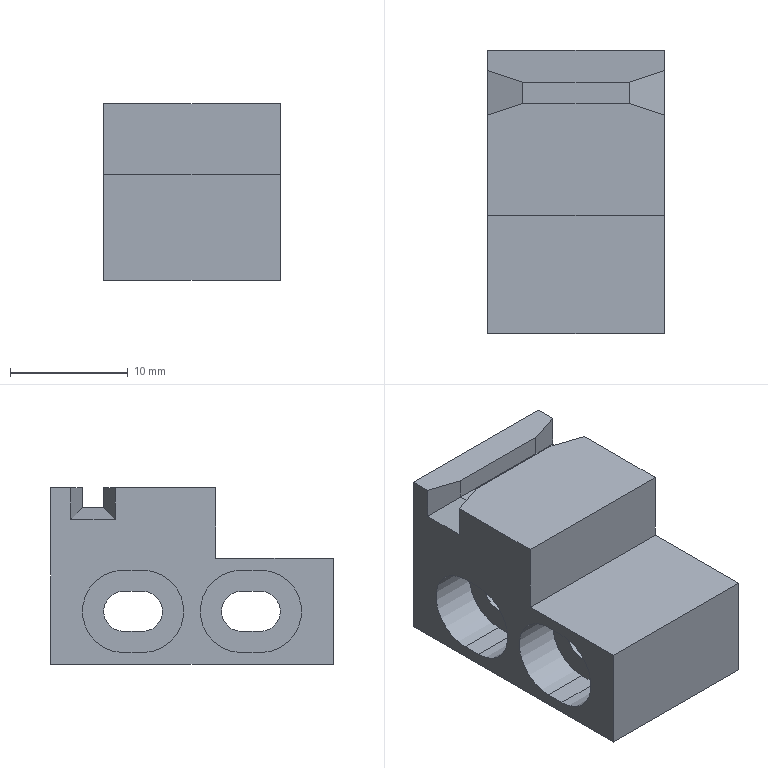Part | NX | features BREP 1 | 1 solid | 48 faces | box 15 x 24 x 15 mm | volume 3436 mm3 | plane 34 | cylinder 14 | commonest cylinder face diameters 7 x10 3.4 x4
STEP:
#1=CARTESIAN_POINT('',(-8.,-13.5,1.5));
#2=VERTEX_POINT('',#1);
#3=CARTESIAN_POINT('',(-8.,-3.5,1.5));
#4=VERTEX_POINT('',#3);
#5=CARTESIAN_POINT('',(-8.,-13.5,1.5));
#6=DIRECTION('',(0.,1.,0.));
#7=VECTOR('',#6,1000.);
#8=LINE('',#5,#7);
#9=EDGE_CURVE('',#2,#4,#8,.T.);
#10=ORIENTED_EDGE('',*,*,#9,.T.);
#11=CARTESIAN_POINT('',(-23.,-3.5,1.5));
#12=VERTEX_POINT('',#11);
#13=CARTESIAN_POINT('',(-23.,-3.5,1.5));
#14=DIRECTION('',(1.,0.,0.));
#15=VECTOR('',#14,1000.);
#16=LINE('',#13,#15);
#17=EDGE_CURVE('',#12,#4,#16,.T.);
#18=ORIENTED_EDGE('',*,*,#17,.F.);
#19=CARTESIAN_POINT('',(-23.,-13.5,1.5));
#20=VERTEX_POINT('',#19);
#21=CARTESIAN_POINT('',(-23.,-13.5,1.5));
#22=DIRECTION('',(0.,1.,0.));
#23=VECTOR('',#22,1000.);
#24=LINE('',#21,#23);
#25=EDGE_CURVE('',#20,#12,#24,.T.);
#26=ORIENTED_EDGE('',*,*,#25,.F.);
#27=CARTESIAN_POINT('',(-23.,-13.5,1.5));
#28=DIRECTION('',(1.,0.,0.));
#29=VECTOR('',#28,1000.);
#30=LINE('',#27,#29);
#31=EDGE_CURVE('',#20,#2,#30,.T.);
#32=ORIENTED_EDGE('',*,*,#31,.T.);
#33=EDGE_LOOP('',(#10,#18,#26,#32));
#34=FACE_BOUND('',#33,.T.);
#35=CARTESIAN_POINT('',(-23.,-13.5,1.5));
#36=DIRECTION('',(0.,0.,-1.));
#37=DIRECTION('',(-1.,0.,0.));
#38=AXIS2_PLACEMENT_3D('',#35,#36,#37);
#39=PLANE('',#38);
#40=ADVANCED_FACE('',(#34),#39,.F.);
#41=CARTESIAN_POINT('',(-8.,-3.5,7.5));
#42=VERTEX_POINT('',#41);
#43=CARTESIAN_POINT('',(-8.,-3.5,7.5));
#44=DIRECTION('',(0.,0.,1.));
#45=VECTOR('',#44,1000.);
#46=LINE('',#43,#45);
#47=EDGE_CURVE('',#4,#42,#46,.T.);
#48=ORIENTED_EDGE('',*,*,#47,.T.);
#49=CARTESIAN_POINT('',(-23.,-3.5,7.5));
#50=VERTEX_POINT('',#49);
#51=CARTESIAN_POINT('',(-23.,-3.5,7.5));
#52=DIRECTION('',(1.,0.,0.));
#53=VECTOR('',#52,1000.);
#54=LINE('',#51,#53);
#55=EDGE_CURVE('',#50,#42,#54,.T.);
#56=ORIENTED_EDGE('',*,*,#55,.F.);
#57=CARTESIAN_POINT('',(-23.,-3.5,7.5));
#58=DIRECTION('',(0.,0.,1.));
#59=VECTOR('',#58,1000.);
#60=LINE('',#57,#59);
#61=EDGE_CURVE('',#12,#50,#60,.T.);
#62=ORIENTED_EDGE('',*,*,#61,.F.);
#63=ORIENTED_EDGE('',*,*,#17,.T.);
#64=EDGE_LOOP('',(#48,#56,#62,#63));
#65=FACE_BOUND('',#64,.T.);
#66=CARTESIAN_POINT('',(-23.,-3.5,7.5));
#67=DIRECTION('',(0.,1.,0.));
#68=DIRECTION('',(-1.,0.,0.));
#69=AXIS2_PLACEMENT_3D('',#66,#67,#68);
#70=PLANE('',#69);
#71=ADVANCED_FACE('',(#65),#70,.F.);
#72=CARTESIAN_POINT('',(-8.,5.,4.8));
#73=VERTEX_POINT('',#72);
#74=CARTESIAN_POINT('',(-11.,6.,5.8));
#75=VERTEX_POINT('',#74);
#76=CARTESIAN_POINT('',(-8.736,5.245,5.045));
#77=DIRECTION('',(-0.9045,0.3015,0.3015));
#78=VECTOR('',#77,1000.);
#79=LINE('',#76,#78);
#80=EDGE_CURVE('',#73,#75,#79,.T.);
#81=ORIENTED_EDGE('',*,*,#80,.T.);
#82=CARTESIAN_POINT('',(-11.,6.,7.5));
#83=VERTEX_POINT('',#82);
#84=CARTESIAN_POINT('',(-11.,6.,5.8));
#85=DIRECTION('',(0.,0.,-1.));
#86=VECTOR('',#85,1000.);
#87=LINE('',#84,#86);
#88=EDGE_CURVE('',#83,#75,#87,.T.);
#89=ORIENTED_EDGE('',*,*,#88,.F.);
#90=CARTESIAN_POINT('',(-8.,5.,7.5));
#91=VERTEX_POINT('',#90);
#92=CARTESIAN_POINT('',(-8.,5.,7.5));
#93=DIRECTION('',(-0.9487,0.3162,0.));
#94=VECTOR('',#93,1000.);
#95=LINE('',#92,#94);
#96=EDGE_CURVE('',#91,#83,#95,.T.);
#97=ORIENTED_EDGE('',*,*,#96,.F.);
#98=CARTESIAN_POINT('',(-8.,5.,7.5));
#99=DIRECTION('',(0.,0.,1.));
#100=VECTOR('',#99,1000.);
#101=LINE('',#98,#100);
#102=EDGE_CURVE('',#73,#91,#101,.T.);
#103=ORIENTED_EDGE('',*,*,#102,.F.);
#104=EDGE_LOOP('',(#81,#89,#97,#103));
#105=FACE_BOUND('',#104,.T.);
#106=CARTESIAN_POINT('',(-8.,5.,7.5));
#107=DIRECTION('',(-0.3162,-0.9487,0.));
#108=DIRECTION('',(0.,0.,1.));
#109=AXIS2_PLACEMENT_3D('',#106,#107,#108);
#110=PLANE('',#109);
#111=ADVANCED_FACE('',(#105),#110,.F.);
#112=CARTESIAN_POINT('',(-8.,8.8,4.8));
#113=VERTEX_POINT('',#112);
#114=CARTESIAN_POINT('',(-11.,7.8,5.8));
#115=VERTEX_POINT('',#114);
#116=CARTESIAN_POINT('',(-11.,7.8,5.8));
#117=DIRECTION('',(-0.9045,-0.3015,0.3015));
#118=VECTOR('',#117,1000.);
#119=LINE('',#116,#118);
#120=EDGE_CURVE('',#113,#115,#119,.T.);
#121=ORIENTED_EDGE('',*,*,#120,.T.);
#122=CARTESIAN_POINT('',(-11.,7.8,5.8));
#123=DIRECTION('',(0.,1.,0.));
#124=VECTOR('',#123,1000.);
#125=LINE('',#122,#124);
#126=EDGE_CURVE('',#75,#115,#125,.T.);
#127=ORIENTED_EDGE('',*,*,#126,.F.);
#128=ORIENTED_EDGE('',*,*,#80,.F.);
#129=CARTESIAN_POINT('',(-8.,6.,4.8));
#130=DIRECTION('',(0.,-1.,0.));
#131=VECTOR('',#130,1000.);
#132=LINE('',#129,#131);
#133=EDGE_CURVE('',#113,#73,#132,.T.);
#134=ORIENTED_EDGE('',*,*,#133,.F.);
#135=EDGE_LOOP('',(#121,#127,#128,#134));
#136=FACE_BOUND('',#135,.T.);
#137=CARTESIAN_POINT('',(-11.,0.,5.8));
#138=DIRECTION('',(0.3162,0.,0.9487));
#139=DIRECTION('',(0.,-1.,0.));
#140=AXIS2_PLACEMENT_3D('',#137,#138,#139);
#141=PLANE('',#140);
#142=ADVANCED_FACE('',(#136),#141,.T.);
#143=CARTESIAN_POINT('',(-11.,7.8,7.5));
#144=VERTEX_POINT('',#143);
#145=CARTESIAN_POINT('',(-8.,8.8,7.5));
#146=VERTEX_POINT('',#145);
#147=CARTESIAN_POINT('',(-11.,7.8,7.5));
#148=DIRECTION('',(0.9487,0.3162,0.));
#149=VECTOR('',#148,1000.);
#150=LINE('',#147,#149);
#151=EDGE_CURVE('',#144,#146,#150,.T.);
#152=ORIENTED_EDGE('',*,*,#151,.F.);
#153=CARTESIAN_POINT('',(-11.,7.8,5.8));
#154=DIRECTION('',(0.,0.,1.));
#155=VECTOR('',#154,1000.);
#156=LINE('',#153,#155);
#157=EDGE_CURVE('',#115,#144,#156,.T.);
#158=ORIENTED_EDGE('',*,*,#157,.F.);
#159=ORIENTED_EDGE('',*,*,#120,.F.);
#160=CARTESIAN_POINT('',(-8.,8.8,7.5));
#161=DIRECTION('',(0.,0.,-1.));
#162=VECTOR('',#161,1000.);
#163=LINE('',#160,#162);
#164=EDGE_CURVE('',#146,#113,#163,.T.);
#165=ORIENTED_EDGE('',*,*,#164,.F.);
#166=EDGE_LOOP('',(#152,#158,#159,#165));
#167=FACE_BOUND('',#166,.T.);
#168=CARTESIAN_POINT('',(-11.,7.8,5.8));
#169=DIRECTION('',(-0.3162,0.9487,0.));
#170=DIRECTION('',(0.,0.,1.));
#171=AXIS2_PLACEMENT_3D('',#168,#169,#170);
#172=PLANE('',#171);
#173=ADVANCED_FACE('',(#167),#172,.F.);
#174=CARTESIAN_POINT('',(-8.,4.3,0.5));
#175=VERTEX_POINT('',#174);
#176=CARTESIAN_POINT('',(-8.,2.7,0.5));
#177=VERTEX_POINT('',#176);
#178=CARTESIAN_POINT('',(-8.,2.7,0.5));
#179=DIRECTION('',(0.,-1.,0.));
#180=VECTOR('',#179,1000.);
#181=LINE('',#178,#180);
#182=EDGE_CURVE('',#175,#177,#181,.T.);
#183=ORIENTED_EDGE('',*,*,#182,.T.);
#184=CARTESIAN_POINT('',(-12.,2.7,0.5));
#185=VERTEX_POINT('',#184);
#186=CARTESIAN_POINT('',(-12.,2.7,0.5));
#187=DIRECTION('',(1.,0.,0.));
#188=VECTOR('',#187,1000.);
#189=LINE('',#186,#188);
#190=EDGE_CURVE('',#185,#177,#189,.T.);
#191=ORIENTED_EDGE('',*,*,#190,.F.);
#192=CARTESIAN_POINT('',(-12.,4.3,0.5));
#193=VERTEX_POINT('',#192);
#194=CARTESIAN_POINT('',(-12.,2.7,0.5));
#195=DIRECTION('',(0.,-1.,0.));
#196=VECTOR('',#195,1000.);
#197=LINE('',#194,#196);
#198=EDGE_CURVE('',#193,#185,#197,.T.);
#199=ORIENTED_EDGE('',*,*,#198,.F.);
#200=CARTESIAN_POINT('',(-12.,4.3,0.5));
#201=DIRECTION('',(1.,0.,0.));
#202=VECTOR('',#201,1000.);
#203=LINE('',#200,#202);
#204=EDGE_CURVE('',#193,#175,#203,.T.);
#205=ORIENTED_EDGE('',*,*,#204,.T.);
#206=EDGE_LOOP('',(#183,#191,#199,#205));
#207=FACE_BOUND('',#206,.T.);
#208=CARTESIAN_POINT('',(-12.,2.7,0.5));
#209=DIRECTION('',(0.,0.,1.));
#210=DIRECTION('',(1.,0.,0.));
#211=AXIS2_PLACEMENT_3D('',#208,#209,#210);
#212=PLANE('',#211);
#213=ADVANCED_FACE('',(#207),#212,.F.);
#214=CARTESIAN_POINT('',(-8.,2.7,-6.5));
#215=VERTEX_POINT('',#214);
#216=CARTESIAN_POINT('',(-8.,2.7,-3.));
#217=DIRECTION('',(1.,0.,0.));
#218=DIRECTION('',(0.,1.,0.));
#219=AXIS2_PLACEMENT_3D('',#216,#217,#218);
#220=CIRCLE('',#219,3.5);
#221=EDGE_CURVE('',#177,#215,#220,.T.);
#222=ORIENTED_EDGE('',*,*,#221,.T.);
#223=CARTESIAN_POINT('',(-12.,2.7,-6.5));
#224=VERTEX_POINT('',#223);
#225=CARTESIAN_POINT('',(-12.,2.7,-6.5));
#226=DIRECTION('',(1.,0.,0.));
#227=VECTOR('',#226,1000.);
#228=LINE('',#225,#227);
#229=EDGE_CURVE('',#224,#215,#228,.T.);
#230=ORIENTED_EDGE('',*,*,#229,.F.);
#231=CARTESIAN_POINT('',(-12.,2.7,-3.));
#232=DIRECTION('',(1.,0.,0.));
#233=DIRECTION('',(0.,1.,0.));
#234=AXIS2_PLACEMENT_3D('',#231,#232,#233);
#235=CIRCLE('',#234,3.5);
#236=EDGE_CURVE('',#185,#224,#235,.T.);
#237=ORIENTED_EDGE('',*,*,#236,.F.);
#238=ORIENTED_EDGE('',*,*,#190,.T.);
#239=EDGE_LOOP('',(#222,#230,#237,#238));
#240=FACE_BOUND('',#239,.T.);
#241=CARTESIAN_POINT('',(-12.,2.7,-3.));
#242=DIRECTION('',(1.,0.,0.));
#243=DIRECTION('',(0.,1.,0.));
#244=AXIS2_PLACEMENT_3D('',#241,#242,#243);
#245=CYLINDRICAL_SURFACE('',#244,3.5);
#246=ADVANCED_FACE('',(#240),#245,.F.);
#247=CARTESIAN_POINT('',(-8.,4.3,-6.5));
#248=VERTEX_POINT('',#247);
#249=CARTESIAN_POINT('',(-8.,4.3,-6.5));
#250=DIRECTION('',(0.,1.,0.));
#251=VECTOR('',#250,1000.);
#252=LINE('',#249,#251);
#253=EDGE_CURVE('',#215,#248,#252,.T.);
#254=ORIENTED_EDGE('',*,*,#253,.T.);
#255=CARTESIAN_POINT('',(-12.,4.3,-6.5));
#256=VERTEX_POINT('',#255);
#257=CARTESIAN_POINT('',(-12.,4.3,-6.5));
#258=DIRECTION('',(1.,0.,0.));
#259=VECTOR('',#258,1000.);
#260=LINE('',#257,#259);
#261=EDGE_CURVE('',#256,#248,#260,.T.);
#262=ORIENTED_EDGE('',*,*,#261,.F.);
#263=CARTESIAN_POINT('',(-12.,4.3,-6.5));
#264=DIRECTION('',(0.,1.,0.));
#265=VECTOR('',#264,1000.);
#266=LINE('',#263,#265);
#267=EDGE_CURVE('',#224,#256,#266,.T.);
#268=ORIENTED_EDGE('',*,*,#267,.F.);
#269=ORIENTED_EDGE('',*,*,#229,.T.);
#270=EDGE_LOOP('',(#254,#262,#268,#269));
#271=FACE_BOUND('',#270,.T.);
#272=CARTESIAN_POINT('',(-12.,4.3,-6.5));
#273=DIRECTION('',(0.,0.,-1.));
#274=DIRECTION('',(-1.,0.,0.));
#275=AXIS2_PLACEMENT_3D('',#272,#273,#274);
#276=PLANE('',#275);
#277=ADVANCED_FACE('',(#271),#276,.F.);
#278=CARTESIAN_POINT('',(-12.,7.8,-3.));
#279=VERTEX_POINT('',#278);
#280=CARTESIAN_POINT('',(-8.,7.8,-3.));
#281=VERTEX_POINT('',#280);
#282=CARTESIAN_POINT('',(-12.,7.8,-3.));
#283=DIRECTION('',(1.,0.,0.));
#284=VECTOR('',#283,1000.);
#285=LINE('',#282,#284);
#286=EDGE_CURVE('',#279,#281,#285,.T.);
#287=ORIENTED_EDGE('',*,*,#286,.F.);
#288=CARTESIAN_POINT('',(-12.,4.3,-3.));
#289=DIRECTION('',(1.,0.,0.));
#290=DIRECTION('',(0.,1.,0.));
#291=AXIS2_PLACEMENT_3D('',#288,#289,#290);
#292=CIRCLE('',#291,3.5);
#293=EDGE_CURVE('',#256,#279,#292,.T.);
#294=ORIENTED_EDGE('',*,*,#293,.F.);
#295=ORIENTED_EDGE('',*,*,#261,.T.);
#296=CARTESIAN_POINT('',(-8.,4.3,-3.));
#297=DIRECTION('',(1.,0.,0.));
#298=DIRECTION('',(0.,1.,0.));
#299=AXIS2_PLACEMENT_3D('',#296,#297,#298);
#300=CIRCLE('',#299,3.5);
#301=EDGE_CURVE('',#248,#281,#300,.T.);
#302=ORIENTED_EDGE('',*,*,#301,.T.);
#303=EDGE_LOOP('',(#287,#294,#295,#302));
#304=FACE_BOUND('',#303,.T.);
#305=CARTESIAN_POINT('',(-12.,4.3,-3.));
#306=DIRECTION('',(1.,0.,0.));
#307=DIRECTION('',(0.,1.,0.));
#308=AXIS2_PLACEMENT_3D('',#305,#306,#307);
#309=CYLINDRICAL_SURFACE('',#308,3.5);
#310=ADVANCED_FACE('',(#304),#309,.F.);
#311=CARTESIAN_POINT('',(-12.,4.3,-4.7));
#312=VERTEX_POINT('',#311);
#313=CARTESIAN_POINT('',(-12.,2.7,-4.7));
#314=VERTEX_POINT('',#313);
#315=CARTESIAN_POINT('',(-12.,2.7,-4.7));
#316=DIRECTION('',(0.,-1.,0.));
#317=VECTOR('',#316,1000.);
#318=LINE('',#315,#317);
#319=EDGE_CURVE('',#312,#314,#318,.T.);
#320=ORIENTED_EDGE('',*,*,#319,.T.);
#321=CARTESIAN_POINT('',(-12.,2.7,-1.3));
#322=VERTEX_POINT('',#321);
#323=CARTESIAN_POINT('',(-12.,2.7,-3.));
#324=DIRECTION('',(-1.,0.,0.));
#325=DIRECTION('',(0.,1.,0.));
#326=AXIS2_PLACEMENT_3D('',#323,#324,#325);
#327=CIRCLE('',#326,1.7);
#328=EDGE_CURVE('',#314,#322,#327,.T.);
#329=ORIENTED_EDGE('',*,*,#328,.T.);
#330=CARTESIAN_POINT('',(-12.,4.3,-1.3));
#331=VERTEX_POINT('',#330);
#332=CARTESIAN_POINT('',(-12.,2.7,-1.3));
#333=DIRECTION('',(0.,1.,0.));
#334=VECTOR('',#333,1000.);
#335=LINE('',#332,#334);
#336=EDGE_CURVE('',#322,#331,#335,.T.);
#337=ORIENTED_EDGE('',*,*,#336,.T.);
#338=CARTESIAN_POINT('',(-12.,4.3,-3.));
#339=DIRECTION('',(-1.,0.,0.));
#340=DIRECTION('',(0.,1.,0.));
#341=AXIS2_PLACEMENT_3D('',#338,#339,#340);
#342=CIRCLE('',#341,1.7);
#343=EDGE_CURVE('',#331,#312,#342,.T.);
#344=ORIENTED_EDGE('',*,*,#343,.T.);
#345=EDGE_LOOP('',(#320,#329,#337,#344));
#346=FACE_BOUND('',#345,.T.);
#347=ORIENTED_EDGE('',*,*,#293,.T.);
#348=CARTESIAN_POINT('',(-12.,4.3,-3.));
#349=DIRECTION('',(1.,0.,0.));
#350=DIRECTION('',(0.,1.,0.));
#351=AXIS2_PLACEMENT_3D('',#348,#349,#350);
#352=CIRCLE('',#351,3.5);
#353=EDGE_CURVE('',#279,#193,#352,.T.);
#354=ORIENTED_EDGE('',*,*,#353,.T.);
#355=ORIENTED_EDGE('',*,*,#198,.T.);
#356=ORIENTED_EDGE('',*,*,#236,.T.);
#357=ORIENTED_EDGE('',*,*,#267,.T.);
#358=EDGE_LOOP('',(#347,#354,#355,#356,#357));
#359=FACE_BOUND('',#358,.T.);
#360=CARTESIAN_POINT('',(-12.,4.3,-3.));
#361=DIRECTION('',(1.,0.,0.));
#362=DIRECTION('',(0.,1.,0.));
#363=AXIS2_PLACEMENT_3D('',#360,#361,#362);
#364=PLANE('',#363);
#365=ADVANCED_FACE('',(#346,#359),#364,.T.);
#366=CARTESIAN_POINT('',(-8.,-5.7,0.5));
#367=VERTEX_POINT('',#366);
#368=CARTESIAN_POINT('',(-8.,-7.3,0.5));
#369=VERTEX_POINT('',#368);
#370=CARTESIAN_POINT('',(-8.,-7.3,0.5));
#371=DIRECTION('',(0.,-1.,0.));
#372=VECTOR('',#371,1000.);
#373=LINE('',#370,#372);
#374=EDGE_CURVE('',#367,#369,#373,.T.);
#375=ORIENTED_EDGE('',*,*,#374,.T.);
#376=CARTESIAN_POINT('',(-12.,-7.3,0.5));
#377=VERTEX_POINT('',#376);
#378=CARTESIAN_POINT('',(-12.,-7.3,0.5));
#379=DIRECTION('',(1.,0.,0.));
#380=VECTOR('',#379,1000.);
#381=LINE('',#378,#380);
#382=EDGE_CURVE('',#377,#369,#381,.T.);
#383=ORIENTED_EDGE('',*,*,#382,.F.);
#384=CARTESIAN_POINT('',(-12.,-5.7,0.5));
#385=VERTEX_POINT('',#384);
#386=CARTESIAN_POINT('',(-12.,-7.3,0.5));
#387=DIRECTION('',(0.,-1.,0.));
#388=VECTOR('',#387,1000.);
#389=LINE('',#386,#388);
#390=EDGE_CURVE('',#385,#377,#389,.T.);
#391=ORIENTED_EDGE('',*,*,#390,.F.);
#392=CARTESIAN_POINT('',(-12.,-5.7,0.5));
#393=DIRECTION('',(1.,0.,0.));
#394=VECTOR('',#393,1000.);
#395=LINE('',#392,#394);
#396=EDGE_CURVE('',#385,#367,#395,.T.);
#397=ORIENTED_EDGE('',*,*,#396,.T.);
#398=EDGE_LOOP('',(#375,#383,#391,#397));
#399=FACE_BOUND('',#398,.T.);
#400=CARTESIAN_POINT('',(-12.,-7.3,0.5));
#401=DIRECTION('',(0.,0.,1.));
#402=DIRECTION('',(1.,0.,0.));
#403=AXIS2_PLACEMENT_3D('',#400,#401,#402);
#404=PLANE('',#403);
#405=ADVANCED_FACE('',(#399),#404,.F.);
#406=CARTESIAN_POINT('',(-8.,-7.3,-6.5));
#407=VERTEX_POINT('',#406);
#408=CARTESIAN_POINT('',(-8.,-7.3,-3.));
#409=DIRECTION('',(1.,0.,0.));
#410=DIRECTION('',(0.,1.,0.));
#411=AXIS2_PLACEMENT_3D('',#408,#409,#410);
#412=CIRCLE('',#411,3.5);
#413=EDGE_CURVE('',#369,#407,#412,.T.);
#414=ORIENTED_EDGE('',*,*,#413,.T.);
#415=CARTESIAN_POINT('',(-12.,-7.3,-6.5));
#416=VERTEX_POINT('',#415);
#417=CARTESIAN_POINT('',(-12.,-7.3,-6.5));
#418=DIRECTION('',(1.,0.,0.));
#419=VECTOR('',#418,1000.);
#420=LINE('',#417,#419);
#421=EDGE_CURVE('',#416,#407,#420,.T.);
#422=ORIENTED_EDGE('',*,*,#421,.F.);
#423=CARTESIAN_POINT('',(-12.,-7.3,-3.));
#424=DIRECTION('',(1.,0.,0.));
#425=DIRECTION('',(0.,1.,0.));
#426=AXIS2_PLACEMENT_3D('',#423,#424,#425);
#427=CIRCLE('',#426,3.5);
#428=EDGE_CURVE('',#377,#416,#427,.T.);
#429=ORIENTED_EDGE('',*,*,#428,.F.);
#430=ORIENTED_EDGE('',*,*,#382,.T.);
#431=EDGE_LOOP('',(#414,#422,#429,#430));
#432=FACE_BOUND('',#431,.T.);
#433=CARTESIAN_POINT('',(-12.,-7.3,-3.));
#434=DIRECTION('',(1.,0.,0.));
#435=DIRECTION('',(0.,1.,0.));
#436=AXIS2_PLACEMENT_3D('',#433,#434,#435);
#437=CYLINDRICAL_SURFACE('',#436,3.5);
#438=ADVANCED_FACE('',(#432),#437,.F.);
#439=CARTESIAN_POINT('',(-8.,-5.7,-6.5));
#440=VERTEX_POINT('',#439);
#441=CARTESIAN_POINT('',(-8.,-5.7,-6.5));
#442=DIRECTION('',(0.,1.,0.));
#443=VECTOR('',#442,1000.);
#444=LINE('',#441,#443);
#445=EDGE_CURVE('',#407,#440,#444,.T.);
#446=ORIENTED_EDGE('',*,*,#445,.T.);
#447=CARTESIAN_POINT('',(-12.,-5.7,-6.5));
#448=VERTEX_POINT('',#447);
#449=CARTESIAN_POINT('',(-12.,-5.7,-6.5));
#450=DIRECTION('',(1.,0.,0.));
#451=VECTOR('',#450,1000.);
#452=LINE('',#449,#451);
#453=EDGE_CURVE('',#448,#440,#452,.T.);
#454=ORIENTED_EDGE('',*,*,#453,.F.);
#455=CARTESIAN_POINT('',(-12.,-5.7,-6.5));
#456=DIRECTION('',(0.,1.,0.));
#457=VECTOR('',#456,1000.);
#458=LINE('',#455,#457);
#459=EDGE_CURVE('',#416,#448,#458,.T.);
#460=ORIENTED_EDGE('',*,*,#459,.F.);
#461=ORIENTED_EDGE('',*,*,#421,.T.);
#462=EDGE_LOOP('',(#446,#454,#460,#461));
#463=FACE_BOUND('',#462,.T.);
#464=CARTESIAN_POINT('',(-12.,-5.7,-6.5));
#465=DIRECTION('',(0.,0.,-1.));
#466=DIRECTION('',(-1.,0.,0.));
#467=AXIS2_PLACEMENT_3D('',#464,#465,#466);
#468=PLANE('',#467);
#469=ADVANCED_FACE('',(#463),#468,.F.);
#470=CARTESIAN_POINT('',(-12.,-2.2,-3.));
#471=VERTEX_POINT('',#470);
#472=CARTESIAN_POINT('',(-8.,-2.2,-3.));
#473=VERTEX_POINT('',#472);
#474=CARTESIAN_POINT('',(-12.,-2.2,-3.));
#475=DIRECTION('',(1.,0.,0.));
#476=VECTOR('',#475,1000.);
#477=LINE('',#474,#476);
#478=EDGE_CURVE('',#471,#473,#477,.T.);
#479=ORIENTED_EDGE('',*,*,#478,.F.);
#480=CARTESIAN_POINT('',(-12.,-5.7,-3.));
#481=DIRECTION('',(1.,0.,0.));
#482=DIRECTION('',(0.,1.,0.));
#483=AXIS2_PLACEMENT_3D('',#480,#481,#482);
#484=CIRCLE('',#483,3.5);
#485=EDGE_CURVE('',#448,#471,#484,.T.);
#486=ORIENTED_EDGE('',*,*,#485,.F.);
#487=ORIENTED_EDGE('',*,*,#453,.T.);
#488=CARTESIAN_POINT('',(-8.,-5.7,-3.));
#489=DIRECTION('',(1.,0.,0.));
#490=DIRECTION('',(0.,1.,0.));
#491=AXIS2_PLACEMENT_3D('',#488,#489,#490);
#492=CIRCLE('',#491,3.5);
#493=EDGE_CURVE('',#440,#473,#492,.T.);
#494=ORIENTED_EDGE('',*,*,#493,.T.);
#495=EDGE_LOOP('',(#479,#486,#487,#494));
#496=FACE_BOUND('',#495,.T.);
#497=CARTESIAN_POINT('',(-12.,-5.7,-3.));
#498=DIRECTION('',(1.,0.,0.));
#499=DIRECTION('',(0.,1.,0.));
#500=AXIS2_PLACEMENT_3D('',#497,#498,#499);
#501=CYLINDRICAL_SURFACE('',#500,3.5);
#502=ADVANCED_FACE('',(#496),#501,.F.);
#503=CARTESIAN_POINT('',(-12.,-5.7,-4.7));
#504=VERTEX_POINT('',#503);
#505=CARTESIAN_POINT('',(-12.,-7.3,-4.7));
#506=VERTEX_POINT('',#505);
#507=CARTESIAN_POINT('',(-12.,-7.3,-4.7));
#508=DIRECTION('',(0.,-1.,0.));
#509=VECTOR('',#508,1000.);
#510=LINE('',#507,#509);
#511=EDGE_CURVE('',#504,#506,#510,.T.);
#512=ORIENTED_EDGE('',*,*,#511,.T.);
#513=CARTESIAN_POINT('',(-12.,-7.3,-1.3));
#514=VERTEX_POINT('',#513);
#515=CARTESIAN_POINT('',(-12.,-7.3,-3.));
#516=DIRECTION('',(-1.,0.,0.));
#517=DIRECTION('',(0.,1.,0.));
#518=AXIS2_PLACEMENT_3D('',#515,#516,#517);
#519=CIRCLE('',#518,1.7);
#520=EDGE_CURVE('',#506,#514,#519,.T.);
#521=ORIENTED_EDGE('',*,*,#520,.T.);
#522=CARTESIAN_POINT('',(-12.,-5.7,-1.3));
#523=VERTEX_POINT('',#522);
#524=CARTESIAN_POINT('',(-12.,-7.3,-1.3));
#525=DIRECTION('',(0.,1.,0.));
#526=VECTOR('',#525,1000.);
#527=LINE('',#524,#526);
#528=EDGE_CURVE('',#514,#523,#527,.T.);
#529=ORIENTED_EDGE('',*,*,#528,.T.);
#530=CARTESIAN_POINT('',(-12.,-5.7,-3.));
#531=DIRECTION('',(-1.,0.,0.));
#532=DIRECTION('',(0.,1.,0.));
#533=AXIS2_PLACEMENT_3D('',#530,#531,#532);
#534=CIRCLE('',#533,1.7);
#535=EDGE_CURVE('',#523,#504,#534,.T.);
#536=ORIENTED_EDGE('',*,*,#535,.T.);
#537=EDGE_LOOP('',(#512,#521,#529,#536));
#538=FACE_BOUND('',#537,.T.);
#539=ORIENTED_EDGE('',*,*,#485,.T.);
#540=CARTESIAN_POINT('',(-12.,-5.7,-3.));
#541=DIRECTION('',(1.,0.,0.));
#542=DIRECTION('',(0.,1.,0.));
#543=AXIS2_PLACEMENT_3D('',#540,#541,#542);
#544=CIRCLE('',#543,3.5);
#545=EDGE_CURVE('',#471,#385,#544,.T.);
#546=ORIENTED_EDGE('',*,*,#545,.T.);
#547=ORIENTED_EDGE('',*,*,#390,.T.);
#548=ORIENTED_EDGE('',*,*,#428,.T.);
#549=ORIENTED_EDGE('',*,*,#459,.T.);
#550=EDGE_LOOP('',(#539,#546,#547,#548,#549));
#551=FACE_BOUND('',#550,.T.);
#552=CARTESIAN_POINT('',(-12.,-5.7,-3.));
#553=DIRECTION('',(1.,0.,0.));
#554=DIRECTION('',(0.,1.,0.));
#555=AXIS2_PLACEMENT_3D('',#552,#553,#554);
#556=PLANE('',#555);
#557=ADVANCED_FACE('',(#538,#551),#556,.T.);
#558=CARTESIAN_POINT('',(-23.,-5.7,0.5));
#559=VERTEX_POINT('',#558);
#560=CARTESIAN_POINT('',(-19.,-5.7,0.5));
#561=VERTEX_POINT('',#560);
#562=CARTESIAN_POINT('',(-23.,-5.7,0.5));
#563=DIRECTION('',(1.,0.,0.));
#564=VECTOR('',#563,1000.);
#565=LINE('',#562,#564);
#566=EDGE_CURVE('',#559,#561,#565,.T.);
#567=ORIENTED_EDGE('',*,*,#566,.T.);
#568=CARTESIAN_POINT('',(-19.,-7.3,0.5));
#569=VERTEX_POINT('',#568);
#570=CARTESIAN_POINT('',(-19.,-7.3,0.5));
#571=DIRECTION('',(0.,1.,0.));
#572=VECTOR('',#571,1000.);
#573=LINE('',#570,#572);
#574=EDGE_CURVE('',#569,#561,#573,.T.);
#575=ORIENTED_EDGE('',*,*,#574,.F.);
#576=CARTESIAN_POINT('',(-23.,-7.3,0.5));
#577=VERTEX_POINT('',#576);
#578=CARTESIAN_POINT('',(-23.,-7.3,0.5));
#579=DIRECTION('',(-1.,0.,0.));
#580=VECTOR('',#579,1000.);
#581=LINE('',#578,#580);
#582=EDGE_CURVE('',#569,#577,#581,.T.);
#583=ORIENTED_EDGE('',*,*,#582,.T.);
#584=CARTESIAN_POINT('',(-23.,-7.3,0.5));
#585=DIRECTION('',(0.,1.,0.));
#586=VECTOR('',#585,1000.);
#587=LINE('',#584,#586);
#588=EDGE_CURVE('',#577,#559,#587,.T.);
#589=ORIENTED_EDGE('',*,*,#588,.T.);
#590=EDGE_LOOP('',(#567,#575,#583,#589));
#591=FACE_BOUND('',#590,.T.);
#592=CARTESIAN_POINT('',(-23.,-7.3,0.5));
#593=DIRECTION('',(0.,0.,1.));
#594=DIRECTION('',(1.,0.,0.));
#595=AXIS2_PLACEMENT_3D('',#592,#593,#594);
#596=PLANE('',#595);
#597=ADVANCED_FACE('',(#591),#596,.F.);
#598=CARTESIAN_POINT('',(-19.,-5.7,-6.5));
#599=VERTEX_POINT('',#598);
#600=CARTESIAN_POINT('',(-23.,-5.7,-6.5));
#601=VERTEX_POINT('',#600);
#602=CARTESIAN_POINT('',(-23.,-5.7,-6.5));
#603=DIRECTION('',(-1.,0.,0.));
#604=VECTOR('',#603,1000.);
#605=LINE('',#602,#604);
#606=EDGE_CURVE('',#599,#601,#605,.T.);
#607=ORIENTED_EDGE('',*,*,#606,.T.);
#608=CARTESIAN_POINT('',(-23.,-7.3,-6.5));
#609=VERTEX_POINT('',#608);
#610=CARTESIAN_POINT('',(-23.,-7.3,-6.5));
#611=DIRECTION('',(0.,1.,0.));
#612=VECTOR('',#611,1000.);
#613=LINE('',#610,#612);
#614=EDGE_CURVE('',#609,#601,#613,.T.);
#615=ORIENTED_EDGE('',*,*,#614,.F.);
#616=CARTESIAN_POINT('',(-19.,-7.3,-6.5));
#617=VERTEX_POINT('',#616);
#618=CARTESIAN_POINT('',(-23.,-7.3,-6.5));
#619=DIRECTION('',(1.,0.,0.));
#620=VECTOR('',#619,1000.);
#621=LINE('',#618,#620);
#622=EDGE_CURVE('',#609,#617,#621,.T.);
#623=ORIENTED_EDGE('',*,*,#622,.T.);
#624=CARTESIAN_POINT('',(-19.,-7.3,-6.5));
#625=DIRECTION('',(0.,1.,0.));
#626=VECTOR('',#625,1000.);
#627=LINE('',#624,#626);
#628=EDGE_CURVE('',#617,#599,#627,.T.);
#629=ORIENTED_EDGE('',*,*,#628,.T.);
#630=EDGE_LOOP('',(#607,#615,#623,#629));
#631=FACE_BOUND('',#630,.T.);
#632=CARTESIAN_POINT('',(-23.,-7.3,-6.5));
#633=DIRECTION('',(0.,0.,-1.));
#634=DIRECTION('',(-1.,0.,0.));
#635=AXIS2_PLACEMENT_3D('',#632,#633,#634);
#636=PLANE('',#635);
#637=ADVANCED_FACE('',(#631),#636,.F.);
#638=CARTESIAN_POINT('',(-23.,-7.3,-3.));
#639=DIRECTION('',(-1.,0.,0.));
#640=DIRECTION('',(0.,0.,1.));
#641=AXIS2_PLACEMENT_3D('',#638,#639,#640);
#642=CIRCLE('',#641,3.5);
#643=EDGE_CURVE('',#609,#577,#642,.T.);
#644=ORIENTED_EDGE('',*,*,#643,.T.);
#645=ORIENTED_EDGE('',*,*,#582,.F.);
#646=CARTESIAN_POINT('',(-19.,-7.3,-3.));
#647=DIRECTION('',(-1.,0.,0.));
#648=DIRECTION('',(0.,0.,1.));
#649=AXIS2_PLACEMENT_3D('',#646,#647,#648);
#650=CIRCLE('',#649,3.5);
#651=EDGE_CURVE('',#617,#569,#650,.T.);
#652=ORIENTED_EDGE('',*,*,#651,.F.);
#653=ORIENTED_EDGE('',*,*,#622,.F.);
#654=EDGE_LOOP('',(#644,#645,#652,#653));
#655=FACE_BOUND('',#654,.T.);
#656=CARTESIAN_POINT('',(-23.,-7.3,-3.));
#657=DIRECTION('',(-1.,0.,0.));
#658=DIRECTION('',(0.,0.,1.));
#659=AXIS2_PLACEMENT_3D('',#656,#657,#658);
#660=CYLINDRICAL_SURFACE('',#659,3.5);
#661=ADVANCED_FACE('',(#655),#660,.F.);
#662=CARTESIAN_POINT('',(-19.,-5.7,-3.));
#663=DIRECTION('',(-1.,0.,0.));
#664=DIRECTION('',(0.,0.,1.));
#665=AXIS2_PLACEMENT_3D('',#662,#663,#664);
#666=CIRCLE('',#665,3.5);
#667=EDGE_CURVE('',#561,#599,#666,.T.);
#668=ORIENTED_EDGE('',*,*,#667,.F.);
#669=ORIENTED_EDGE('',*,*,#566,.F.);
#670=CARTESIAN_POINT('',(-23.,-5.7,-3.));
#671=DIRECTION('',(-1.,0.,0.));
#672=DIRECTION('',(0.,0.,1.));
#673=AXIS2_PLACEMENT_3D('',#670,#671,#672);
#674=CIRCLE('',#673,3.5);
#675=EDGE_CURVE('',#559,#601,#674,.T.);
#676=ORIENTED_EDGE('',*,*,#675,.T.);
#677=ORIENTED_EDGE('',*,*,#606,.F.);
#678=EDGE_LOOP('',(#668,#669,#676,#677));
#679=FACE_BOUND('',#678,.T.);
#680=CARTESIAN_POINT('',(-23.,-5.7,-3.));
#681=DIRECTION('',(-1.,0.,0.));
#682=DIRECTION('',(0.,0.,1.));
#683=AXIS2_PLACEMENT_3D('',#680,#681,#682);
#684=CYLINDRICAL_SURFACE('',#683,3.5);
#685=ADVANCED_FACE('',(#679),#684,.F.);
#686=ORIENTED_EDGE('',*,*,#667,.T.);
#687=ORIENTED_EDGE('',*,*,#628,.F.);
#688=ORIENTED_EDGE('',*,*,#651,.T.);
#689=ORIENTED_EDGE('',*,*,#574,.T.);
#690=EDGE_LOOP('',(#686,#687,#688,#689));
#691=FACE_BOUND('',#690,.T.);
#692=CARTESIAN_POINT('',(-19.,-7.3,-1.3));
#693=VERTEX_POINT('',#692);
#694=CARTESIAN_POINT('',(-19.,-5.7,-1.3));
#695=VERTEX_POINT('',#694);
#696=CARTESIAN_POINT('',(-19.,-7.3,-1.3));
#697=DIRECTION('',(0.,1.,0.));
#698=VECTOR('',#697,1000.);
#699=LINE('',#696,#698);
#700=EDGE_CURVE('',#693,#695,#699,.T.);
#701=ORIENTED_EDGE('',*,*,#700,.F.);
#702=CARTESIAN_POINT('',(-19.,-7.3,-4.7));
#703=VERTEX_POINT('',#702);
#704=CARTESIAN_POINT('',(-19.,-7.3,-3.));
#705=DIRECTION('',(-1.,0.,0.));
#706=DIRECTION('',(0.,0.,1.));
#707=AXIS2_PLACEMENT_3D('',#704,#705,#706);
#708=CIRCLE('',#707,1.7);
#709=EDGE_CURVE('',#703,#693,#708,.T.);
#710=ORIENTED_EDGE('',*,*,#709,.F.);
#711=CARTESIAN_POINT('',(-19.,-5.7,-4.7));
#712=VERTEX_POINT('',#711);
#713=CARTESIAN_POINT('',(-19.,-7.3,-4.7));
#714=DIRECTION('',(0.,1.,0.));
#715=VECTOR('',#714,1000.);
#716=LINE('',#713,#715);
#717=EDGE_CURVE('',#703,#712,#716,.T.);
#718=ORIENTED_EDGE('',*,*,#717,.T.);
#719=CARTESIAN_POINT('',(-19.,-5.7,-3.));
#720=DIRECTION('',(-1.,0.,0.));
#721=DIRECTION('',(0.,0.,1.));
#722=AXIS2_PLACEMENT_3D('',#719,#720,#721);
#723=CIRCLE('',#722,1.7);
#724=EDGE_CURVE('',#695,#712,#723,.T.);
#725=ORIENTED_EDGE('',*,*,#724,.F.);
#726=EDGE_LOOP('',(#701,#710,#718,#725));
#727=FACE_BOUND('',#726,.T.);
#728=CARTESIAN_POINT('',(-19.,-4.,-3.));
#729=DIRECTION('',(1.,0.,0.));
#730=DIRECTION('',(0.,0.,-1.));
#731=AXIS2_PLACEMENT_3D('',#728,#729,#730);
#732=PLANE('',#731);
#733=ADVANCED_FACE('',(#691,#727),#732,.F.);
#734=CARTESIAN_POINT('',(-23.,4.3,0.5));
#735=VERTEX_POINT('',#734);
#736=CARTESIAN_POINT('',(-19.,4.3,0.5));
#737=VERTEX_POINT('',#736);
#738=CARTESIAN_POINT('',(-23.,4.3,0.5));
#739=DIRECTION('',(1.,0.,0.));
#740=VECTOR('',#739,1000.);
#741=LINE('',#738,#740);
#742=EDGE_CURVE('',#735,#737,#741,.T.);
#743=ORIENTED_EDGE('',*,*,#742,.T.);
#744=CARTESIAN_POINT('',(-19.,2.7,0.5));
#745=VERTEX_POINT('',#744);
#746=CARTESIAN_POINT('',(-19.,2.7,0.5));
#747=DIRECTION('',(0.,1.,0.));
#748=VECTOR('',#747,1000.);
#749=LINE('',#746,#748);
#750=EDGE_CURVE('',#745,#737,#749,.T.);
#751=ORIENTED_EDGE('',*,*,#750,.F.);
#752=CARTESIAN_POINT('',(-23.,2.7,0.5));
#753=VERTEX_POINT('',#752);
#754=CARTESIAN_POINT('',(-23.,2.7,0.5));
#755=DIRECTION('',(-1.,0.,0.));
#756=VECTOR('',#755,1000.);
#757=LINE('',#754,#756);
#758=EDGE_CURVE('',#745,#753,#757,.T.);
#759=ORIENTED_EDGE('',*,*,#758,.T.);
#760=CARTESIAN_POINT('',(-23.,2.7,0.5));
#761=DIRECTION('',(0.,1.,0.));
#762=VECTOR('',#761,1000.);
#763=LINE('',#760,#762);
#764=EDGE_CURVE('',#753,#735,#763,.T.);
#765=ORIENTED_EDGE('',*,*,#764,.T.);
#766=EDGE_LOOP('',(#743,#751,#759,#765));
#767=FACE_BOUND('',#766,.T.);
#768=CARTESIAN_POINT('',(-23.,2.7,0.5));
#769=DIRECTION('',(0.,0.,1.));
#770=DIRECTION('',(1.,0.,0.));
#771=AXIS2_PLACEMENT_3D('',#768,#769,#770);
#772=PLANE('',#771);
#773=ADVANCED_FACE('',(#767),#772,.F.);
#774=CARTESIAN_POINT('',(-19.,4.3,-6.5));
#775=VERTEX_POINT('',#774);
#776=CARTESIAN_POINT('',(-23.,4.3,-6.5));
#777=VERTEX_POINT('',#776);
#778=CARTESIAN_POINT('',(-23.,4.3,-6.5));
#779=DIRECTION('',(-1.,0.,0.));
#780=VECTOR('',#779,1000.);
#781=LINE('',#778,#780);
#782=EDGE_CURVE('',#775,#777,#781,.T.);
#783=ORIENTED_EDGE('',*,*,#782,.T.);
#784=CARTESIAN_POINT('',(-23.,2.7,-6.5));
#785=VERTEX_POINT('',#784);
#786=CARTESIAN_POINT('',(-23.,2.7,-6.5));
#787=DIRECTION('',(0.,1.,0.));
#788=VECTOR('',#787,1000.);
#789=LINE('',#786,#788);
#790=EDGE_CURVE('',#785,#777,#789,.T.);
#791=ORIENTED_EDGE('',*,*,#790,.F.);
#792=CARTESIAN_POINT('',(-19.,2.7,-6.5));
#793=VERTEX_POINT('',#792);
#794=CARTESIAN_POINT('',(-23.,2.7,-6.5));
#795=DIRECTION('',(1.,0.,0.));
#796=VECTOR('',#795,1000.);
#797=LINE('',#794,#796);
#798=EDGE_CURVE('',#785,#793,#797,.T.);
#799=ORIENTED_EDGE('',*,*,#798,.T.);
#800=CARTESIAN_POINT('',(-19.,2.7,-6.5));
#801=DIRECTION('',(0.,1.,0.));
#802=VECTOR('',#801,1000.);
#803=LINE('',#800,#802);
#804=EDGE_CURVE('',#793,#775,#803,.T.);
#805=ORIENTED_EDGE('',*,*,#804,.T.);
#806=EDGE_LOOP('',(#783,#791,#799,#805));
#807=FACE_BOUND('',#806,.T.);
#808=CARTESIAN_POINT('',(-23.,2.7,-6.5));
#809=DIRECTION('',(0.,0.,-1.));
#810=DIRECTION('',(-1.,0.,0.));
#811=AXIS2_PLACEMENT_3D('',#808,#809,#810);
#812=PLANE('',#811);
#813=ADVANCED_FACE('',(#807),#812,.F.);
#814=CARTESIAN_POINT('',(-23.,2.7,-3.));
#815=DIRECTION('',(-1.,0.,0.));
#816=DIRECTION('',(0.,0.,1.));
#817=AXIS2_PLACEMENT_3D('',#814,#815,#816);
#818=CIRCLE('',#817,3.5);
#819=EDGE_CURVE('',#785,#753,#818,.T.);
#820=ORIENTED_EDGE('',*,*,#819,.T.);
#821=ORIENTED_EDGE('',*,*,#758,.F.);
#822=CARTESIAN_POINT('',(-19.,2.7,-3.));
#823=DIRECTION('',(-1.,0.,0.));
#824=DIRECTION('',(0.,0.,1.));
#825=AXIS2_PLACEMENT_3D('',#822,#823,#824);
#826=CIRCLE('',#825,3.5);
#827=EDGE_CURVE('',#793,#745,#826,.T.);
#828=ORIENTED_EDGE('',*,*,#827,.F.);
#829=ORIENTED_EDGE('',*,*,#798,.F.);
#830=EDGE_LOOP('',(#820,#821,#828,#829));
#831=FACE_BOUND('',#830,.T.);
#832=CARTESIAN_POINT('',(-23.,2.7,-3.));
#833=DIRECTION('',(-1.,0.,0.));
#834=DIRECTION('',(0.,0.,1.));
#835=AXIS2_PLACEMENT_3D('',#832,#833,#834);
#836=CYLINDRICAL_SURFACE('',#835,3.5);
#837=ADVANCED_FACE('',(#831),#836,.F.);
#838=CARTESIAN_POINT('',(-19.,4.3,-3.));
#839=DIRECTION('',(-1.,0.,0.));
#840=DIRECTION('',(0.,0.,1.));
#841=AXIS2_PLACEMENT_3D('',#838,#839,#840);
#842=CIRCLE('',#841,3.5);
#843=EDGE_CURVE('',#737,#775,#842,.T.);
#844=ORIENTED_EDGE('',*,*,#843,.F.);
#845=ORIENTED_EDGE('',*,*,#742,.F.);
#846=CARTESIAN_POINT('',(-23.,4.3,-3.));
#847=DIRECTION('',(-1.,0.,0.));
#848=DIRECTION('',(0.,0.,1.));
#849=AXIS2_PLACEMENT_3D('',#846,#847,#848);
#850=CIRCLE('',#849,3.5);
#851=EDGE_CURVE('',#735,#777,#850,.T.);
#852=ORIENTED_EDGE('',*,*,#851,.T.);
#853=ORIENTED_EDGE('',*,*,#782,.F.);
#854=EDGE_LOOP('',(#844,#845,#852,#853));
#855=FACE_BOUND('',#854,.T.);
#856=CARTESIAN_POINT('',(-23.,4.3,-3.));
#857=DIRECTION('',(-1.,0.,0.));
#858=DIRECTION('',(0.,0.,1.));
#859=AXIS2_PLACEMENT_3D('',#856,#857,#858);
#860=CYLINDRICAL_SURFACE('',#859,3.5);
#861=ADVANCED_FACE('',(#855),#860,.F.);
#862=ORIENTED_EDGE('',*,*,#843,.T.);
#863=ORIENTED_EDGE('',*,*,#804,.F.);
#864=ORIENTED_EDGE('',*,*,#827,.T.);
#865=ORIENTED_EDGE('',*,*,#750,.T.);
#866=EDGE_LOOP('',(#862,#863,#864,#865));
#867=FACE_BOUND('',#866,.T.);
#868=CARTESIAN_POINT('',(-19.,2.7,-1.3));
#869=VERTEX_POINT('',#868);
#870=CARTESIAN_POINT('',(-19.,4.3,-1.3));
#871=VERTEX_POINT('',#870);
#872=CARTESIAN_POINT('',(-19.,2.7,-1.3));
#873=DIRECTION('',(0.,1.,0.));
#874=VECTOR('',#873,1000.);
#875=LINE('',#872,#874);
#876=EDGE_CURVE('',#869,#871,#875,.T.);
#877=ORIENTED_EDGE('',*,*,#876,.F.);
#878=CARTESIAN_POINT('',(-19.,2.7,-4.7));
#879=VERTEX_POINT('',#878);
#880=CARTESIAN_POINT('',(-19.,2.7,-3.));
#881=DIRECTION('',(-1.,0.,0.));
#882=DIRECTION('',(0.,0.,1.));
#883=AXIS2_PLACEMENT_3D('',#880,#881,#882);
#884=CIRCLE('',#883,1.7);
#885=EDGE_CURVE('',#879,#869,#884,.T.);
#886=ORIENTED_EDGE('',*,*,#885,.F.);
#887=CARTESIAN_POINT('',(-19.,4.3,-4.7));
#888=VERTEX_POINT('',#887);
#889=CARTESIAN_POINT('',(-19.,2.7,-4.7));
#890=DIRECTION('',(0.,1.,0.));
#891=VECTOR('',#890,1000.);
#892=LINE('',#889,#891);
#893=EDGE_CURVE('',#879,#888,#892,.T.);
#894=ORIENTED_EDGE('',*,*,#893,.T.);
#895=CARTESIAN_POINT('',(-19.,4.3,-3.));
#896=DIRECTION('',(-1.,0.,0.));
#897=DIRECTION('',(0.,0.,1.));
#898=AXIS2_PLACEMENT_3D('',#895,#896,#897);
#899=CIRCLE('',#898,1.7);
#900=EDGE_CURVE('',#871,#888,#899,.T.);
#901=ORIENTED_EDGE('',*,*,#900,.F.);
#902=EDGE_LOOP('',(#877,#886,#894,#901));
#903=FACE_BOUND('',#902,.T.);
#904=CARTESIAN_POINT('',(-19.,6.,-3.));
#905=DIRECTION('',(1.,0.,0.));
#906=DIRECTION('',(0.,0.,-1.));
#907=AXIS2_PLACEMENT_3D('',#904,#905,#906);
#908=PLANE('',#907);
#909=ADVANCED_FACE('',(#867,#903),#908,.F.);
#910=CARTESIAN_POINT('',(-20.,6.,5.8));
#911=VERTEX_POINT('',#910);
#912=CARTESIAN_POINT('',(-23.,5.,4.8));
#913=VERTEX_POINT('',#912);
#914=CARTESIAN_POINT('',(-20.,6.,5.8));
#915=DIRECTION('',(-0.9045,-0.3015,-0.3015));
#916=VECTOR('',#915,1000.);
#917=LINE('',#914,#916);
#918=EDGE_CURVE('',#911,#913,#917,.T.);
#919=ORIENTED_EDGE('',*,*,#918,.T.);
#920=CARTESIAN_POINT('',(-23.,5.,7.5));
#921=VERTEX_POINT('',#920);
#922=CARTESIAN_POINT('',(-23.,5.,7.5));
#923=DIRECTION('',(0.,0.,-1.));
#924=VECTOR('',#923,1000.);
#925=LINE('',#922,#924);
#926=EDGE_CURVE('',#921,#913,#925,.T.);
#927=ORIENTED_EDGE('',*,*,#926,.F.);
#928=CARTESIAN_POINT('',(-20.,6.,7.5));
#929=VERTEX_POINT('',#928);
#930=CARTESIAN_POINT('',(-20.,6.,7.5));
#931=DIRECTION('',(-0.9487,-0.3162,0.));
#932=VECTOR('',#931,1000.);
#933=LINE('',#930,#932);
#934=EDGE_CURVE('',#929,#921,#933,.T.);
#935=ORIENTED_EDGE('',*,*,#934,.F.);
#936=CARTESIAN_POINT('',(-20.,6.,5.8));
#937=DIRECTION('',(0.,0.,1.));
#938=VECTOR('',#937,1000.);
#939=LINE('',#936,#938);
#940=EDGE_CURVE('',#911,#929,#939,.T.);
#941=ORIENTED_EDGE('',*,*,#940,.F.);
#942=EDGE_LOOP('',(#919,#927,#935,#941));
#943=FACE_BOUND('',#942,.T.);
#944=CARTESIAN_POINT('',(-20.,6.,5.8));
#945=DIRECTION('',(0.3162,-0.9487,0.));
#946=DIRECTION('',(0.,0.,1.));
#947=AXIS2_PLACEMENT_3D('',#944,#945,#946);
#948=PLANE('',#947);
#949=ADVANCED_FACE('',(#943),#948,.F.);
#950=CARTESIAN_POINT('',(-20.,7.8,5.8));
#951=VERTEX_POINT('',#950);
#952=CARTESIAN_POINT('',(-23.,8.8,4.8));
#953=VERTEX_POINT('',#952);
#954=CARTESIAN_POINT('',(-17.873,7.091,6.509));
#955=DIRECTION('',(-0.9045,0.3015,-0.3015));
#956=VECTOR('',#955,1000.);
#957=LINE('',#954,#956);
#958=EDGE_CURVE('',#951,#953,#957,.T.);
#959=ORIENTED_EDGE('',*,*,#958,.T.);
#960=CARTESIAN_POINT('',(-23.,7.8,4.8));
#961=DIRECTION('',(0.,1.,0.));
#962=VECTOR('',#961,1000.);
#963=LINE('',#960,#962);
#964=EDGE_CURVE('',#913,#953,#963,.T.);
#965=ORIENTED_EDGE('',*,*,#964,.F.);
#966=ORIENTED_EDGE('',*,*,#918,.F.);
#967=CARTESIAN_POINT('',(-20.,6.,5.8));
#968=DIRECTION('',(0.,-1.,0.));
#969=VECTOR('',#968,1000.);
#970=LINE('',#967,#969);
#971=EDGE_CURVE('',#951,#911,#970,.T.);
#972=ORIENTED_EDGE('',*,*,#971,.F.);
#973=EDGE_LOOP('',(#959,#965,#966,#972));
#974=FACE_BOUND('',#973,.T.);
#975=CARTESIAN_POINT('',(-20.,0.,5.8));
#976=DIRECTION('',(-0.3162,0.,0.9487));
#977=DIRECTION('',(0.,1.,0.));
#978=AXIS2_PLACEMENT_3D('',#975,#976,#977);
#979=PLANE('',#978);
#980=ADVANCED_FACE('',(#974),#979,.T.);
#981=CARTESIAN_POINT('',(-23.,8.8,7.5));
#982=VERTEX_POINT('',#981);
#983=CARTESIAN_POINT('',(-20.,7.8,7.5));
#984=VERTEX_POINT('',#983);
#985=CARTESIAN_POINT('',(-23.,8.8,7.5));
#986=DIRECTION('',(0.9487,-0.3162,0.));
#987=VECTOR('',#986,1000.);
#988=LINE('',#985,#987);
#989=EDGE_CURVE('',#982,#984,#988,.T.);
#990=ORIENTED_EDGE('',*,*,#989,.F.);
#991=CARTESIAN_POINT('',(-23.,8.8,7.5));
#992=DIRECTION('',(0.,0.,1.));
#993=VECTOR('',#992,1000.);
#994=LINE('',#991,#993);
#995=EDGE_CURVE('',#953,#982,#994,.T.);
#996=ORIENTED_EDGE('',*,*,#995,.F.);
#997=ORIENTED_EDGE('',*,*,#958,.F.);
#998=CARTESIAN_POINT('',(-20.,7.8,5.8));
#999=DIRECTION('',(0.,0.,-1.));
#1000=VECTOR('',#999,1000.);
#1001=LINE('',#998,#1000);
#1002=EDGE_CURVE('',#984,#951,#1001,.T.);
#1003=ORIENTED_EDGE('',*,*,#1002,.F.);
#1004=EDGE_LOOP('',(#990,#996,#997,#1003));
#1005=FACE_BOUND('',#1004,.T.);
#1006=CARTESIAN_POINT('',(-23.,8.8,7.5));
#1007=DIRECTION('',(0.3162,0.9487,0.));
#1008=DIRECTION('',(0.,0.,1.));
#1009=AXIS2_PLACEMENT_3D('',#1006,#1007,#1008);
#1010=PLANE('',#1009);
#1011=ADVANCED_FACE('',(#1005),#1010,.F.);
#1012=CARTESIAN_POINT('',(-23.,6.,5.8));
#1013=DIRECTION('',(1.,0.,0.));
#1014=VECTOR('',#1013,1000.);
#1015=LINE('',#1012,#1014);
#1016=EDGE_CURVE('',#911,#75,#1015,.T.);
#1017=ORIENTED_EDGE('',*,*,#1016,.T.);
#1018=ORIENTED_EDGE('',*,*,#126,.T.);
#1019=CARTESIAN_POINT('',(-23.,7.8,5.8));
#1020=DIRECTION('',(-1.,0.,0.));
#1021=VECTOR('',#1020,1000.);
#1022=LINE('',#1019,#1021);
#1023=EDGE_CURVE('',#115,#951,#1022,.T.);
#1024=ORIENTED_EDGE('',*,*,#1023,.T.);
#1025=ORIENTED_EDGE('',*,*,#971,.T.);
#1026=EDGE_LOOP('',(#1017,#1018,#1024,#1025));
#1027=FACE_BOUND('',#1026,.T.);
#1028=CARTESIAN_POINT('',(0.,0.,5.8));
#1029=DIRECTION('',(0.,0.,1.));
#1030=DIRECTION('',(1.,0.,0.));
#1031=AXIS2_PLACEMENT_3D('',#1028,#1029,#1030);
#1032=PLANE('',#1031);
#1033=ADVANCED_FACE('',(#1027),#1032,.T.);
#1034=CARTESIAN_POINT('',(-23.,6.,7.5));
#1035=DIRECTION('',(1.,0.,0.));
#1036=VECTOR('',#1035,1000.);
#1037=LINE('',#1034,#1036);
#1038=EDGE_CURVE('',#929,#83,#1037,.T.);
#1039=ORIENTED_EDGE('',*,*,#1038,.T.);
#1040=ORIENTED_EDGE('',*,*,#88,.T.);
#1041=ORIENTED_EDGE('',*,*,#1016,.F.);
#1042=ORIENTED_EDGE('',*,*,#940,.T.);
#1043=EDGE_LOOP('',(#1039,#1040,#1041,#1042));
#1044=FACE_BOUND('',#1043,.T.);
#1045=CARTESIAN_POINT('',(-23.,6.,5.8));
#1046=DIRECTION('',(0.,-1.,0.));
#1047=DIRECTION('',(1.,0.,0.));
#1048=AXIS2_PLACEMENT_3D('',#1045,#1046,#1047);
#1049=PLANE('',#1048);
#1050=ADVANCED_FACE('',(#1044),#1049,.F.);
#1051=ORIENTED_EDGE('',*,*,#1023,.F.);
#1052=ORIENTED_EDGE('',*,*,#157,.T.);
#1053=CARTESIAN_POINT('',(-23.,7.8,7.5));
#1054=DIRECTION('',(-1.,0.,0.));
#1055=VECTOR('',#1054,1000.);
#1056=LINE('',#1053,#1055);
#1057=EDGE_CURVE('',#144,#984,#1056,.T.);
#1058=ORIENTED_EDGE('',*,*,#1057,.T.);
#1059=ORIENTED_EDGE('',*,*,#1002,.T.);
#1060=EDGE_LOOP('',(#1051,#1052,#1058,#1059));
#1061=FACE_BOUND('',#1060,.T.);
#1062=CARTESIAN_POINT('',(-23.,7.8,5.8));
#1063=DIRECTION('',(0.,1.,0.));
#1064=DIRECTION('',(0.,0.,1.));
#1065=AXIS2_PLACEMENT_3D('',#1062,#1063,#1064);
#1066=PLANE('',#1065);
#1067=ADVANCED_FACE('',(#1061),#1066,.F.);
#1068=CARTESIAN_POINT('',(-8.,10.5,-7.5));
#1069=VERTEX_POINT('',#1068);
#1070=CARTESIAN_POINT('',(-23.,10.5,-7.5));
#1071=VERTEX_POINT('',#1070);
#1072=CARTESIAN_POINT('',(-23.,10.5,-7.5));
#1073=DIRECTION('',(-1.,0.,0.));
#1074=VECTOR('',#1073,1000.);
#1075=LINE('',#1072,#1074);
#1076=EDGE_CURVE('',#1069,#1071,#1075,.T.);
#1077=ORIENTED_EDGE('',*,*,#1076,.F.);
#1078=CARTESIAN_POINT('',(-8.,-13.5,-7.5));
#1079=VERTEX_POINT('',#1078);
#1080=CARTESIAN_POINT('',(-8.,10.5,-7.5));
#1081=DIRECTION('',(0.,1.,0.));
#1082=VECTOR('',#1081,1000.);
#1083=LINE('',#1080,#1082);
#1084=EDGE_CURVE('',#1079,#1069,#1083,.T.);
#1085=ORIENTED_EDGE('',*,*,#1084,.F.);
#1086=CARTESIAN_POINT('',(-23.,-13.5,-7.5));
#1087=VERTEX_POINT('',#1086);
#1088=CARTESIAN_POINT('',(-8.,-13.5,-7.5));
#1089=DIRECTION('',(1.,0.,0.));
#1090=VECTOR('',#1089,1000.);
#1091=LINE('',#1088,#1090);
#1092=EDGE_CURVE('',#1087,#1079,#1091,.T.);
#1093=ORIENTED_EDGE('',*,*,#1092,.F.);
#1094=CARTESIAN_POINT('',(-23.,-13.5,-7.5));
#1095=DIRECTION('',(0.,-1.,0.));
#1096=VECTOR('',#1095,1000.);
#1097=LINE('',#1094,#1096);
#1098=EDGE_CURVE('',#1071,#1087,#1097,.T.);
#1099=ORIENTED_EDGE('',*,*,#1098,.F.);
#1100=EDGE_LOOP('',(#1077,#1085,#1093,#1099));
#1101=FACE_BOUND('',#1100,.T.);
#1102=CARTESIAN_POINT('',(0.,0.,-7.5));
#1103=DIRECTION('',(0.,0.,-1.));
#1104=DIRECTION('',(-1.,0.,0.));
#1105=AXIS2_PLACEMENT_3D('',#1102,#1103,#1104);
#1106=PLANE('',#1105);
#1107=ADVANCED_FACE('',(#1101),#1106,.T.);
#1108=CARTESIAN_POINT('',(-23.,-13.5,7.5));
#1109=DIRECTION('',(0.,-1.,0.));
#1110=VECTOR('',#1109,1000.);
#1111=LINE('',#1108,#1110);
#1112=EDGE_CURVE('',#921,#50,#1111,.T.);
#1113=ORIENTED_EDGE('',*,*,#1112,.T.);
#1114=ORIENTED_EDGE('',*,*,#55,.T.);
#1115=CARTESIAN_POINT('',(-8.,10.5,7.5));
#1116=DIRECTION('',(0.,1.,0.));
#1117=VECTOR('',#1116,1000.);
#1118=LINE('',#1115,#1117);
#1119=EDGE_CURVE('',#42,#91,#1118,.T.);
#1120=ORIENTED_EDGE('',*,*,#1119,.T.);
#1121=ORIENTED_EDGE('',*,*,#96,.T.);
#1122=ORIENTED_EDGE('',*,*,#1038,.F.);
#1123=ORIENTED_EDGE('',*,*,#934,.T.);
#1124=EDGE_LOOP('',(#1113,#1114,#1120,#1121,#1122,#1123));
#1125=FACE_BOUND('',#1124,.T.);
#1126=CARTESIAN_POINT('',(0.,0.,7.5));
#1127=DIRECTION('',(0.,0.,-1.));
#1128=DIRECTION('',(-1.,0.,0.));
#1129=AXIS2_PLACEMENT_3D('',#1126,#1127,#1128);
#1130=PLANE('',#1129);
#1131=ADVANCED_FACE('',(#1125),#1130,.F.);
#1132=ORIENTED_EDGE('',*,*,#1119,.F.);
#1133=ORIENTED_EDGE('',*,*,#47,.F.);
#1134=ORIENTED_EDGE('',*,*,#9,.F.);
#1135=CARTESIAN_POINT('',(-8.,-13.5,7.5));
#1136=DIRECTION('',(0.,0.,-1.));
#1137=VECTOR('',#1136,1000.);
#1138=LINE('',#1135,#1137);
#1139=EDGE_CURVE('',#2,#1079,#1138,.T.);
#1140=ORIENTED_EDGE('',*,*,#1139,.T.);
#1141=ORIENTED_EDGE('',*,*,#1084,.T.);
#1142=CARTESIAN_POINT('',(-8.,10.5,7.5));
#1143=VERTEX_POINT('',#1142);
#1144=CARTESIAN_POINT('',(-8.,10.5,7.5));
#1145=DIRECTION('',(0.,0.,-1.));
#1146=VECTOR('',#1145,1000.);
#1147=LINE('',#1144,#1146);
#1148=EDGE_CURVE('',#1143,#1069,#1147,.T.);
#1149=ORIENTED_EDGE('',*,*,#1148,.F.);
#1150=CARTESIAN_POINT('',(-8.,10.5,7.5));
#1151=DIRECTION('',(0.,1.,0.));
#1152=VECTOR('',#1151,1000.);
#1153=LINE('',#1150,#1152);
#1154=EDGE_CURVE('',#146,#1143,#1153,.T.);
#1155=ORIENTED_EDGE('',*,*,#1154,.F.);
#1156=ORIENTED_EDGE('',*,*,#164,.T.);
#1157=ORIENTED_EDGE('',*,*,#133,.T.);
#1158=ORIENTED_EDGE('',*,*,#102,.T.);
#1159=EDGE_LOOP('',(#1132,#1133,#1134,#1140,#1141,#1149,#1155,#1156,#1157,#1158));
#1160=FACE_BOUND('',#1159,.T.);
#1161=ORIENTED_EDGE('',*,*,#374,.F.);
#1162=CARTESIAN_POINT('',(-8.,-5.7,-3.));
#1163=DIRECTION('',(1.,0.,0.));
#1164=DIRECTION('',(0.,1.,0.));
#1165=AXIS2_PLACEMENT_3D('',#1162,#1163,#1164);
#1166=CIRCLE('',#1165,3.5);
#1167=EDGE_CURVE('',#473,#367,#1166,.T.);
#1168=ORIENTED_EDGE('',*,*,#1167,.F.);
#1169=ORIENTED_EDGE('',*,*,#493,.F.);
#1170=ORIENTED_EDGE('',*,*,#445,.F.);
#1171=ORIENTED_EDGE('',*,*,#413,.F.);
#1172=EDGE_LOOP('',(#1161,#1168,#1169,#1170,#1171));
#1173=FACE_BOUND('',#1172,.T.);
#1174=ORIENTED_EDGE('',*,*,#182,.F.);
#1175=CARTESIAN_POINT('',(-8.,4.3,-3.));
#1176=DIRECTION('',(1.,0.,0.));
#1177=DIRECTION('',(0.,1.,0.));
#1178=AXIS2_PLACEMENT_3D('',#1175,#1176,#1177);
#1179=CIRCLE('',#1178,3.5);
#1180=EDGE_CURVE('',#281,#175,#1179,.T.);
#1181=ORIENTED_EDGE('',*,*,#1180,.F.);
#1182=ORIENTED_EDGE('',*,*,#301,.F.);
#1183=ORIENTED_EDGE('',*,*,#253,.F.);
#1184=ORIENTED_EDGE('',*,*,#221,.F.);
#1185=EDGE_LOOP('',(#1174,#1181,#1182,#1183,#1184));
#1186=FACE_BOUND('',#1185,.T.);
#1187=CARTESIAN_POINT('',(-8.,10.5,7.5));
#1188=DIRECTION('',(-1.,0.,0.));
#1189=DIRECTION('',(0.,-1.,0.));
#1190=AXIS2_PLACEMENT_3D('',#1187,#1188,#1189);
#1191=PLANE('',#1190);
#1192=ADVANCED_FACE('',(#1160,#1173,#1186),#1191,.F.);
#1193=ORIENTED_EDGE('',*,*,#1139,.F.);
#1194=ORIENTED_EDGE('',*,*,#31,.F.);
#1195=CARTESIAN_POINT('',(-23.,-13.5,7.5));
#1196=DIRECTION('',(0.,0.,-1.));
#1197=VECTOR('',#1196,1000.);
#1198=LINE('',#1195,#1197);
#1199=EDGE_CURVE('',#20,#1087,#1198,.T.);
#1200=ORIENTED_EDGE('',*,*,#1199,.T.);
#1201=ORIENTED_EDGE('',*,*,#1092,.T.);
#1202=EDGE_LOOP('',(#1193,#1194,#1200,#1201));
#1203=FACE_BOUND('',#1202,.T.);
#1204=CARTESIAN_POINT('',(-8.,-13.5,7.5));
#1205=DIRECTION('',(0.,1.,0.));
#1206=DIRECTION('',(-1.,0.,0.));
#1207=AXIS2_PLACEMENT_3D('',#1204,#1205,#1206);
#1208=PLANE('',#1207);
#1209=ADVANCED_FACE('',(#1203),#1208,.F.);
#1210=ORIENTED_EDGE('',*,*,#25,.T.);
#1211=ORIENTED_EDGE('',*,*,#61,.T.);
#1212=ORIENTED_EDGE('',*,*,#1112,.F.);
#1213=ORIENTED_EDGE('',*,*,#926,.T.);
#1214=ORIENTED_EDGE('',*,*,#964,.T.);
#1215=ORIENTED_EDGE('',*,*,#995,.T.);
#1216=CARTESIAN_POINT('',(-23.,10.5,7.5));
#1217=VERTEX_POINT('',#1216);
#1218=CARTESIAN_POINT('',(-23.,-13.5,7.5));
#1219=DIRECTION('',(0.,-1.,0.));
#1220=VECTOR('',#1219,1000.);
#1221=LINE('',#1218,#1220);
#1222=EDGE_CURVE('',#1217,#982,#1221,.T.);
#1223=ORIENTED_EDGE('',*,*,#1222,.F.);
#1224=CARTESIAN_POINT('',(-23.,10.5,7.5));
#1225=DIRECTION('',(0.,0.,-1.));
#1226=VECTOR('',#1225,1000.);
#1227=LINE('',#1224,#1226);
#1228=EDGE_CURVE('',#1217,#1071,#1227,.T.);
#1229=ORIENTED_EDGE('',*,*,#1228,.T.);
#1230=ORIENTED_EDGE('',*,*,#1098,.T.);
#1231=ORIENTED_EDGE('',*,*,#1199,.F.);
#1232=EDGE_LOOP('',(#1210,#1211,#1212,#1213,#1214,#1215,#1223,#1229,#1230,#1231));
#1233=FACE_BOUND('',#1232,.T.);
#1234=ORIENTED_EDGE('',*,*,#819,.F.);
#1235=ORIENTED_EDGE('',*,*,#790,.T.);
#1236=ORIENTED_EDGE('',*,*,#851,.F.);
#1237=ORIENTED_EDGE('',*,*,#764,.F.);
#1238=EDGE_LOOP('',(#1234,#1235,#1236,#1237));
#1239=FACE_BOUND('',#1238,.T.);
#1240=ORIENTED_EDGE('',*,*,#614,.T.);
#1241=ORIENTED_EDGE('',*,*,#675,.F.);
#1242=ORIENTED_EDGE('',*,*,#588,.F.);
#1243=ORIENTED_EDGE('',*,*,#643,.F.);
#1244=EDGE_LOOP('',(#1240,#1241,#1242,#1243));
#1245=FACE_BOUND('',#1244,.T.);
#1246=CARTESIAN_POINT('',(-23.,-13.5,7.5));
#1247=DIRECTION('',(1.,0.,0.));
#1248=DIRECTION('',(0.,0.,-1.));
#1249=AXIS2_PLACEMENT_3D('',#1246,#1247,#1248);
#1250=PLANE('',#1249);
#1251=ADVANCED_FACE('',(#1233,#1239,#1245),#1250,.F.);
#1252=ORIENTED_EDGE('',*,*,#1076,.T.);
#1253=ORIENTED_EDGE('',*,*,#1228,.F.);
#1254=CARTESIAN_POINT('',(-23.,10.5,7.5));
#1255=DIRECTION('',(-1.,0.,0.));
#1256=VECTOR('',#1255,1000.);
#1257=LINE('',#1254,#1256);
#1258=EDGE_CURVE('',#1143,#1217,#1257,.T.);
#1259=ORIENTED_EDGE('',*,*,#1258,.F.);
#1260=ORIENTED_EDGE('',*,*,#1148,.T.);
#1261=EDGE_LOOP('',(#1252,#1253,#1259,#1260));
#1262=FACE_BOUND('',#1261,.T.);
#1263=CARTESIAN_POINT('',(-23.,10.5,7.5));
#1264=DIRECTION('',(0.,-1.,0.));
#1265=DIRECTION('',(0.,0.,-1.));
#1266=AXIS2_PLACEMENT_3D('',#1263,#1264,#1265);
#1267=PLANE('',#1266);
#1268=ADVANCED_FACE('',(#1262),#1267,.F.);
#1269=ORIENTED_EDGE('',*,*,#1057,.F.);
#1270=ORIENTED_EDGE('',*,*,#151,.T.);
#1271=ORIENTED_EDGE('',*,*,#1154,.T.);
#1272=ORIENTED_EDGE('',*,*,#1258,.T.);
#1273=ORIENTED_EDGE('',*,*,#1222,.T.);
#1274=ORIENTED_EDGE('',*,*,#989,.T.);
#1275=EDGE_LOOP('',(#1269,#1270,#1271,#1272,#1273,#1274));
#1276=FACE_BOUND('',#1275,.T.);
#1277=CARTESIAN_POINT('',(0.,0.,7.5));
#1278=DIRECTION('',(0.,0.,-1.));
#1279=DIRECTION('',(-1.,0.,0.));
#1280=AXIS2_PLACEMENT_3D('',#1277,#1278,#1279);
#1281=PLANE('',#1280);
#1282=ADVANCED_FACE('',(#1276),#1281,.F.);
#1283=ORIENTED_EDGE('',*,*,#528,.F.);
#1284=CARTESIAN_POINT('',(-23.,-7.3,-1.3));
#1285=DIRECTION('',(-1.,0.,0.));
#1286=VECTOR('',#1285,1000.);
#1287=LINE('',#1284,#1286);
#1288=EDGE_CURVE('',#514,#693,#1287,.T.);
#1289=ORIENTED_EDGE('',*,*,#1288,.T.);
#1290=ORIENTED_EDGE('',*,*,#700,.T.);
#1291=CARTESIAN_POINT('',(-23.,-5.7,-1.3));
#1292=DIRECTION('',(1.,0.,0.));
#1293=VECTOR('',#1292,1000.);
#1294=LINE('',#1291,#1293);
#1295=EDGE_CURVE('',#695,#523,#1294,.T.);
#1296=ORIENTED_EDGE('',*,*,#1295,.T.);
#1297=EDGE_LOOP('',(#1283,#1289,#1290,#1296));
#1298=FACE_BOUND('',#1297,.T.);
#1299=CARTESIAN_POINT('',(-23.,-7.3,-1.3));
#1300=DIRECTION('',(0.,0.,1.));
#1301=DIRECTION('',(1.,0.,0.));
#1302=AXIS2_PLACEMENT_3D('',#1299,#1300,#1301);
#1303=PLANE('',#1302);
#1304=ADVANCED_FACE('',(#1298),#1303,.F.);
#1305=ORIENTED_EDGE('',*,*,#511,.F.);
#1306=CARTESIAN_POINT('',(-23.,-5.7,-4.7));
#1307=DIRECTION('',(-1.,0.,0.));
#1308=VECTOR('',#1307,1000.);
#1309=LINE('',#1306,#1308);
#1310=EDGE_CURVE('',#504,#712,#1309,.T.);
#1311=ORIENTED_EDGE('',*,*,#1310,.T.);
#1312=ORIENTED_EDGE('',*,*,#717,.F.);
#1313=CARTESIAN_POINT('',(-23.,-7.3,-4.7));
#1314=DIRECTION('',(1.,0.,0.));
#1315=VECTOR('',#1314,1000.);
#1316=LINE('',#1313,#1315);
#1317=EDGE_CURVE('',#703,#506,#1316,.T.);
#1318=ORIENTED_EDGE('',*,*,#1317,.T.);
#1319=EDGE_LOOP('',(#1305,#1311,#1312,#1318));
#1320=FACE_BOUND('',#1319,.T.);
#1321=CARTESIAN_POINT('',(-23.,-7.3,-4.7));
#1322=DIRECTION('',(0.,0.,-1.));
#1323=DIRECTION('',(-1.,0.,0.));
#1324=AXIS2_PLACEMENT_3D('',#1321,#1322,#1323);
#1325=PLANE('',#1324);
#1326=ADVANCED_FACE('',(#1320),#1325,.F.);
#1327=ORIENTED_EDGE('',*,*,#520,.F.);
#1328=ORIENTED_EDGE('',*,*,#1317,.F.);
#1329=ORIENTED_EDGE('',*,*,#709,.T.);
#1330=ORIENTED_EDGE('',*,*,#1288,.F.);
#1331=EDGE_LOOP('',(#1327,#1328,#1329,#1330));
#1332=FACE_BOUND('',#1331,.T.);
#1333=CARTESIAN_POINT('',(-23.,-7.3,-3.));
#1334=DIRECTION('',(-1.,0.,0.));
#1335=DIRECTION('',(0.,0.,1.));
#1336=AXIS2_PLACEMENT_3D('',#1333,#1334,#1335);
#1337=CYLINDRICAL_SURFACE('',#1336,1.7);
#1338=ADVANCED_FACE('',(#1332),#1337,.F.);
#1339=ORIENTED_EDGE('',*,*,#535,.F.);
#1340=ORIENTED_EDGE('',*,*,#1295,.F.);
#1341=ORIENTED_EDGE('',*,*,#724,.T.);
#1342=ORIENTED_EDGE('',*,*,#1310,.F.);
#1343=EDGE_LOOP('',(#1339,#1340,#1341,#1342));
#1344=FACE_BOUND('',#1343,.T.);
#1345=CARTESIAN_POINT('',(-23.,-5.7,-3.));
#1346=DIRECTION('',(-1.,0.,0.));
#1347=DIRECTION('',(0.,0.,1.));
#1348=AXIS2_PLACEMENT_3D('',#1345,#1346,#1347);
#1349=CYLINDRICAL_SURFACE('',#1348,1.7);
#1350=ADVANCED_FACE('',(#1344),#1349,.F.);
#1351=ORIENTED_EDGE('',*,*,#336,.F.);
#1352=CARTESIAN_POINT('',(-23.,2.7,-1.3));
#1353=DIRECTION('',(-1.,0.,0.));
#1354=VECTOR('',#1353,1000.);
#1355=LINE('',#1352,#1354);
#1356=EDGE_CURVE('',#322,#869,#1355,.T.);
#1357=ORIENTED_EDGE('',*,*,#1356,.T.);
#1358=ORIENTED_EDGE('',*,*,#876,.T.);
#1359=CARTESIAN_POINT('',(-23.,4.3,-1.3));
#1360=DIRECTION('',(1.,0.,0.));
#1361=VECTOR('',#1360,1000.);
#1362=LINE('',#1359,#1361);
#1363=EDGE_CURVE('',#871,#331,#1362,.T.);
#1364=ORIENTED_EDGE('',*,*,#1363,.T.);
#1365=EDGE_LOOP('',(#1351,#1357,#1358,#1364));
#1366=FACE_BOUND('',#1365,.T.);
#1367=CARTESIAN_POINT('',(-23.,2.7,-1.3));
#1368=DIRECTION('',(0.,0.,1.));
#1369=DIRECTION('',(1.,0.,0.));
#1370=AXIS2_PLACEMENT_3D('',#1367,#1368,#1369);
#1371=PLANE('',#1370);
#1372=ADVANCED_FACE('',(#1366),#1371,.F.);
#1373=ORIENTED_EDGE('',*,*,#319,.F.);
#1374=CARTESIAN_POINT('',(-23.,4.3,-4.7));
#1375=DIRECTION('',(-1.,0.,0.));
#1376=VECTOR('',#1375,1000.);
#1377=LINE('',#1374,#1376);
#1378=EDGE_CURVE('',#312,#888,#1377,.T.);
#1379=ORIENTED_EDGE('',*,*,#1378,.T.);
#1380=ORIENTED_EDGE('',*,*,#893,.F.);
#1381=CARTESIAN_POINT('',(-23.,2.7,-4.7));
#1382=DIRECTION('',(1.,0.,0.));
#1383=VECTOR('',#1382,1000.);
#1384=LINE('',#1381,#1383);
#1385=EDGE_CURVE('',#879,#314,#1384,.T.);
#1386=ORIENTED_EDGE('',*,*,#1385,.T.);
#1387=EDGE_LOOP('',(#1373,#1379,#1380,#1386));
#1388=FACE_BOUND('',#1387,.T.);
#1389=CARTESIAN_POINT('',(-23.,2.7,-4.7));
#1390=DIRECTION('',(0.,0.,-1.));
#1391=DIRECTION('',(-1.,0.,0.));
#1392=AXIS2_PLACEMENT_3D('',#1389,#1390,#1391);
#1393=PLANE('',#1392);
#1394=ADVANCED_FACE('',(#1388),#1393,.F.);
#1395=ORIENTED_EDGE('',*,*,#328,.F.);
#1396=ORIENTED_EDGE('',*,*,#1385,.F.);
#1397=ORIENTED_EDGE('',*,*,#885,.T.);
#1398=ORIENTED_EDGE('',*,*,#1356,.F.);
#1399=EDGE_LOOP('',(#1395,#1396,#1397,#1398));
#1400=FACE_BOUND('',#1399,.T.);
#1401=CARTESIAN_POINT('',(-23.,2.7,-3.));
#1402=DIRECTION('',(-1.,0.,0.));
#1403=DIRECTION('',(0.,0.,1.));
#1404=AXIS2_PLACEMENT_3D('',#1401,#1402,#1403);
#1405=CYLINDRICAL_SURFACE('',#1404,1.7);
#1406=ADVANCED_FACE('',(#1400),#1405,.F.);
#1407=ORIENTED_EDGE('',*,*,#343,.F.);
#1408=ORIENTED_EDGE('',*,*,#1363,.F.);
#1409=ORIENTED_EDGE('',*,*,#900,.T.);
#1410=ORIENTED_EDGE('',*,*,#1378,.F.);
#1411=EDGE_LOOP('',(#1407,#1408,#1409,#1410));
#1412=FACE_BOUND('',#1411,.T.);
#1413=CARTESIAN_POINT('',(-23.,4.3,-3.));
#1414=DIRECTION('',(-1.,0.,0.));
#1415=DIRECTION('',(0.,0.,1.));
#1416=AXIS2_PLACEMENT_3D('',#1413,#1414,#1415);
#1417=CYLINDRICAL_SURFACE('',#1416,1.7);
#1418=ADVANCED_FACE('',(#1412),#1417,.F.);
#1419=ORIENTED_EDGE('',*,*,#545,.F.);
#1420=ORIENTED_EDGE('',*,*,#478,.T.);
#1421=ORIENTED_EDGE('',*,*,#1167,.T.);
#1422=ORIENTED_EDGE('',*,*,#396,.F.);
#1423=EDGE_LOOP('',(#1419,#1420,#1421,#1422));
#1424=FACE_BOUND('',#1423,.T.);
#1425=CARTESIAN_POINT('',(-12.,-5.7,-3.));
#1426=DIRECTION('',(1.,0.,0.));
#1427=DIRECTION('',(0.,1.,0.));
#1428=AXIS2_PLACEMENT_3D('',#1425,#1426,#1427);
#1429=CYLINDRICAL_SURFACE('',#1428,3.5);
#1430=ADVANCED_FACE('',(#1424),#1429,.F.);
#1431=ORIENTED_EDGE('',*,*,#353,.F.);
#1432=ORIENTED_EDGE('',*,*,#286,.T.);
#1433=ORIENTED_EDGE('',*,*,#1180,.T.);
#1434=ORIENTED_EDGE('',*,*,#204,.F.);
#1435=EDGE_LOOP('',(#1431,#1432,#1433,#1434));
#1436=FACE_BOUND('',#1435,.T.);
#1437=CARTESIAN_POINT('',(-12.,4.3,-3.));
#1438=DIRECTION('',(1.,0.,0.));
#1439=DIRECTION('',(0.,1.,0.));
#1440=AXIS2_PLACEMENT_3D('',#1437,#1438,#1439);
#1441=CYLINDRICAL_SURFACE('',#1440,3.5);
#1442=ADVANCED_FACE('',(#1436),#1441,.F.);
#1443=CLOSED_SHELL('',(#40,#71,#111,#142,#173,#213,#246,#277,#310,#365,#405,#438,#469,#502,#557,#597,#637,#661,#685,#733,#773,#813,#837,#861,#909,#949,#980,#1011,#1033,#1050,#1067,#1107,#1131,#1192,#1209,#1251,#1268,#1282,#1304,#1326,#1338,#1350,#1372,#1394,#1406,#1418,#1430,#1442));
#1444=MANIFOLD_SOLID_BREP('',#1443);
#1445=(LENGTH_UNIT()NAMED_UNIT(*)SI_UNIT(.MILLI.,.METRE.));
#1446=UNCERTAINTY_MEASURE_WITH_UNIT(LENGTH_MEASURE(0.00001),#1445,'','');
#1447=(NAMED_UNIT(*)PLANE_ANGLE_UNIT()SI_UNIT($,.RADIAN.));
#1448=(NAMED_UNIT(*)SI_UNIT($,.STERADIAN.)SOLID_ANGLE_UNIT());
#1449=(GEOMETRIC_REPRESENTATION_CONTEXT(3)GLOBAL_UNCERTAINTY_ASSIGNED_CONTEXT((#1446))GLOBAL_UNIT_ASSIGNED_CONTEXT((#1445,#1447,#1448))REPRESENTATION_CONTEXT('',''));
#1450=ADVANCED_BREP_SHAPE_REPRESENTATION('',(#1444),#1449);